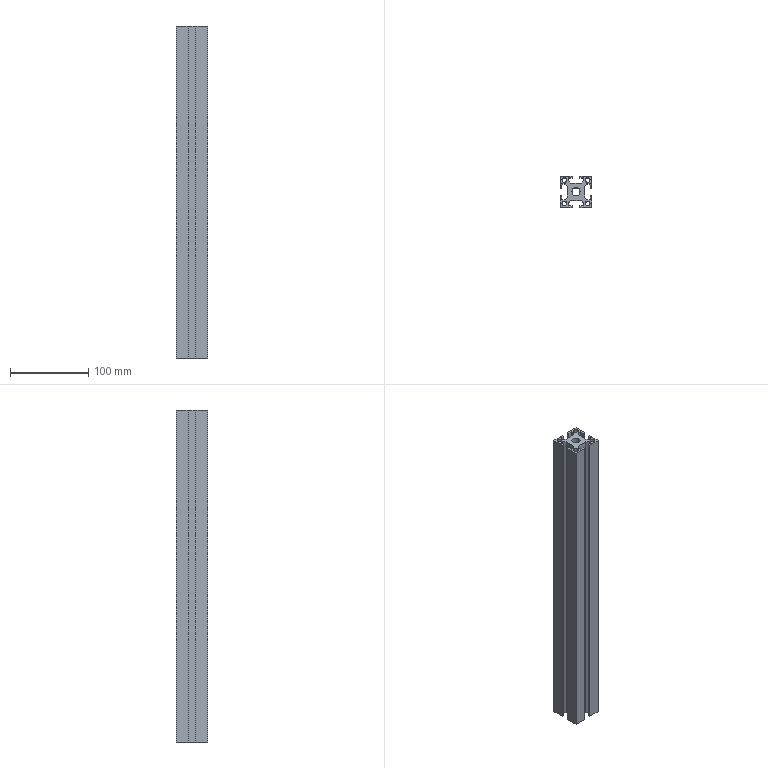Part | SolidWorks | features BaseBody 1 | 1 solid | 56 faces | box 40 x 40 x 425 mm | volume 338433 mm3 | plane 46 | cylinder 10 | commonest cylinder face diameters 6 x8 10.5 x2